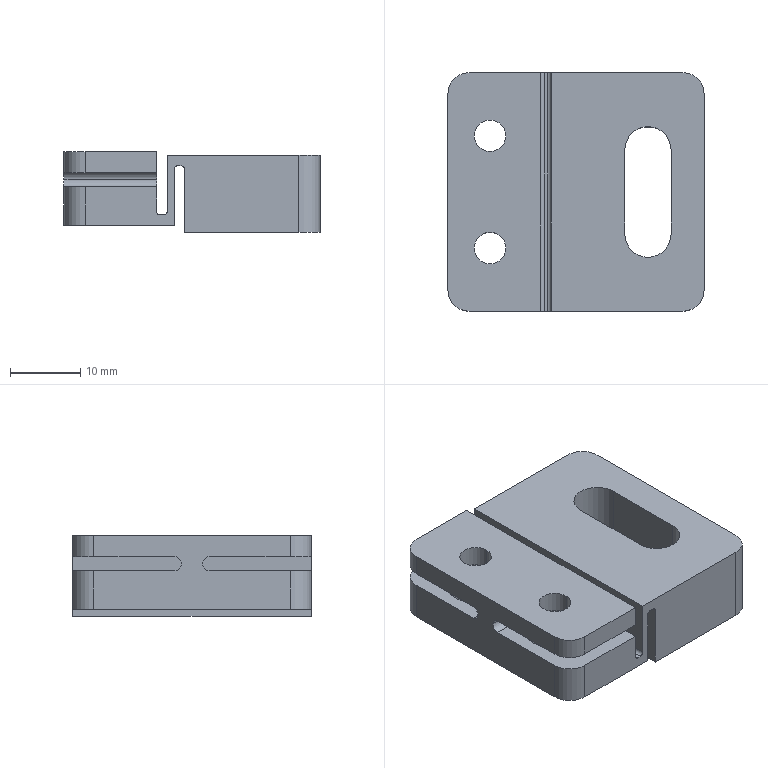Part | SolidWorks | features ICE 13, MoveFace 5, Fillet 3, DelFace 2, Extrusion 1, PLine 1 | 1 solid | 46 faces | box 36.5 x 34 x 11.5 mm | volume 9581 mm3 | cylinder 24 | plane 22 | commonest cylinder face diameters 6 x6 1 x4 2 x4 4.5 x4 8.5 x4 6.6 x2
STEP:
#1=CARTESIAN_POINT('',(-4.75,8.,6.5));
#2=VERTEX_POINT('',#1);
#3=CARTESIAN_POINT('',(-13.25,8.,6.5));
#4=VERTEX_POINT('',#3);
#5=CARTESIAN_POINT('',(-9.,8.,6.5));
#6=DIRECTION('',(0.,0.,-1.));
#7=DIRECTION('',(-1.,0.,0.));
#8=AXIS2_PLACEMENT_3D('',#5,#6,#7);
#9=CIRCLE('',#8,4.25);
#10=EDGE_CURVE('',#2,#4,#9,.T.);
#11=ORIENTED_EDGE('',*,*,#10,.F.);
#12=CARTESIAN_POINT('',(-4.75,8.,1.));
#13=VERTEX_POINT('',#12);
#14=CARTESIAN_POINT('',(-4.75,8.,7.5));
#15=DIRECTION('',(0.,0.,-1.));
#16=VECTOR('',#15,1000.);
#17=LINE('',#14,#16);
#18=EDGE_CURVE('',#2,#13,#17,.T.);
#19=ORIENTED_EDGE('',*,*,#18,.T.);
#20=CARTESIAN_POINT('',(-13.25,8.,1.));
#21=VERTEX_POINT('',#20);
#22=CARTESIAN_POINT('',(-9.,8.,1.));
#23=DIRECTION('',(0.,0.,-1.));
#24=DIRECTION('',(-1.,0.,0.));
#25=AXIS2_PLACEMENT_3D('',#22,#23,#24);
#26=CIRCLE('',#25,4.25);
#27=EDGE_CURVE('',#13,#21,#26,.T.);
#28=ORIENTED_EDGE('',*,*,#27,.T.);
#29=CARTESIAN_POINT('',(-13.25,8.,7.5));
#30=DIRECTION('',(0.,0.,-1.));
#31=VECTOR('',#30,1000.);
#32=LINE('',#29,#31);
#33=EDGE_CURVE('',#4,#21,#32,.T.);
#34=ORIENTED_EDGE('',*,*,#33,.F.);
#35=EDGE_LOOP('',(#11,#19,#28,#34));
#36=FACE_OUTER_BOUND('',#35,.T.);
#37=CARTESIAN_POINT('',(-9.,8.,7.5));
#38=DIRECTION('',(0.,0.,-1.));
#39=DIRECTION('',(-1.,0.,0.));
#40=AXIS2_PLACEMENT_3D('',#37,#38,#39);
#41=CYLINDRICAL_SURFACE('',#40,4.25);
#42=ADVANCED_FACE('',(#36),#41,.F.);
#43=CARTESIAN_POINT('',(-4.75,-8.,6.5));
#44=VERTEX_POINT('',#43);
#45=CARTESIAN_POINT('',(-13.25,-8.,6.5));
#46=VERTEX_POINT('',#45);
#47=CARTESIAN_POINT('',(-9.,-8.,6.5));
#48=DIRECTION('',(0.,0.,-1.));
#49=DIRECTION('',(-1.,0.,0.));
#50=AXIS2_PLACEMENT_3D('',#47,#48,#49);
#51=CIRCLE('',#50,4.25);
#52=EDGE_CURVE('',#44,#46,#51,.T.);
#53=ORIENTED_EDGE('',*,*,#52,.F.);
#54=CARTESIAN_POINT('',(-4.75,-8.,1.));
#55=VERTEX_POINT('',#54);
#56=CARTESIAN_POINT('',(-4.75,-8.,7.5));
#57=DIRECTION('',(0.,0.,-1.));
#58=VECTOR('',#57,1000.);
#59=LINE('',#56,#58);
#60=EDGE_CURVE('',#44,#55,#59,.T.);
#61=ORIENTED_EDGE('',*,*,#60,.T.);
#62=CARTESIAN_POINT('',(-13.25,-8.,1.));
#63=VERTEX_POINT('',#62);
#64=CARTESIAN_POINT('',(-9.,-8.,1.));
#65=DIRECTION('',(0.,0.,-1.));
#66=DIRECTION('',(-1.,0.,0.));
#67=AXIS2_PLACEMENT_3D('',#64,#65,#66);
#68=CIRCLE('',#67,4.25);
#69=EDGE_CURVE('',#55,#63,#68,.T.);
#70=ORIENTED_EDGE('',*,*,#69,.T.);
#71=CARTESIAN_POINT('',(-13.25,-8.,7.5));
#72=DIRECTION('',(0.,0.,-1.));
#73=VECTOR('',#72,1000.);
#74=LINE('',#71,#73);
#75=EDGE_CURVE('',#46,#63,#74,.T.);
#76=ORIENTED_EDGE('',*,*,#75,.F.);
#77=EDGE_LOOP('',(#53,#61,#70,#76));
#78=FACE_OUTER_BOUND('',#77,.T.);
#79=CARTESIAN_POINT('',(-9.,-8.,7.5));
#80=DIRECTION('',(0.,0.,-1.));
#81=DIRECTION('',(-1.,0.,0.));
#82=AXIS2_PLACEMENT_3D('',#79,#80,#81);
#83=CYLINDRICAL_SURFACE('',#82,4.25);
#84=ADVANCED_FACE('',(#78),#83,.F.);
#85=CARTESIAN_POINT('',(-11.25,8.,8.5));
#86=VERTEX_POINT('',#85);
#87=CARTESIAN_POINT('',(-6.75,8.,8.5));
#88=VERTEX_POINT('',#87);
#89=CARTESIAN_POINT('',(-9.,8.,8.5));
#90=DIRECTION('',(0.,0.,1.));
#91=DIRECTION('',(0.,-1.,0.));
#92=AXIS2_PLACEMENT_3D('',#89,#90,#91);
#93=CIRCLE('',#92,2.25);
#94=EDGE_CURVE('',#86,#88,#93,.T.);
#95=ORIENTED_EDGE('',*,*,#94,.F.);
#96=CARTESIAN_POINT('',(-11.25,8.,11.5));
#97=VERTEX_POINT('',#96);
#98=CARTESIAN_POINT('',(-11.25,8.,-6.364));
#99=DIRECTION('',(0.,0.,1.));
#100=VECTOR('',#99,1000.);
#101=LINE('',#98,#100);
#102=EDGE_CURVE('',#86,#97,#101,.T.);
#103=ORIENTED_EDGE('',*,*,#102,.T.);
#104=CARTESIAN_POINT('',(-6.75,8.,11.5));
#105=VERTEX_POINT('',#104);
#106=CARTESIAN_POINT('',(-9.,8.,11.5));
#107=DIRECTION('',(0.,0.,1.));
#108=DIRECTION('',(1.,0.,0.));
#109=AXIS2_PLACEMENT_3D('',#106,#107,#108);
#110=CIRCLE('',#109,2.25);
#111=EDGE_CURVE('',#97,#105,#110,.T.);
#112=ORIENTED_EDGE('',*,*,#111,.T.);
#113=CARTESIAN_POINT('',(-6.75,8.,-6.364));
#114=DIRECTION('',(0.,0.,1.));
#115=VECTOR('',#114,1000.);
#116=LINE('',#113,#115);
#117=EDGE_CURVE('',#88,#105,#116,.T.);
#118=ORIENTED_EDGE('',*,*,#117,.F.);
#119=EDGE_LOOP('',(#95,#103,#112,#118));
#120=FACE_OUTER_BOUND('',#119,.T.);
#121=CARTESIAN_POINT('',(-9.,8.,-6.364));
#122=DIRECTION('',(0.,0.,1.));
#123=DIRECTION('',(1.,0.,0.));
#124=AXIS2_PLACEMENT_3D('',#121,#122,#123);
#125=CYLINDRICAL_SURFACE('',#124,2.25);
#126=ADVANCED_FACE('',(#120),#125,.F.);
#127=CARTESIAN_POINT('',(-11.25,-8.,8.5));
#128=VERTEX_POINT('',#127);
#129=CARTESIAN_POINT('',(-6.75,-8.,8.5));
#130=VERTEX_POINT('',#129);
#131=CARTESIAN_POINT('',(-9.,-8.,8.5));
#132=DIRECTION('',(0.,0.,1.));
#133=DIRECTION('',(0.,-1.,0.));
#134=AXIS2_PLACEMENT_3D('',#131,#132,#133);
#135=CIRCLE('',#134,2.25);
#136=EDGE_CURVE('',#128,#130,#135,.T.);
#137=ORIENTED_EDGE('',*,*,#136,.F.);
#138=CARTESIAN_POINT('',(-11.25,-8.,11.5));
#139=VERTEX_POINT('',#138);
#140=CARTESIAN_POINT('',(-11.25,-8.,-6.364));
#141=DIRECTION('',(0.,0.,1.));
#142=VECTOR('',#141,1000.);
#143=LINE('',#140,#142);
#144=EDGE_CURVE('',#128,#139,#143,.T.);
#145=ORIENTED_EDGE('',*,*,#144,.T.);
#146=CARTESIAN_POINT('',(-6.75,-8.,11.5));
#147=VERTEX_POINT('',#146);
#148=CARTESIAN_POINT('',(-9.,-8.,11.5));
#149=DIRECTION('',(0.,0.,1.));
#150=DIRECTION('',(1.,0.,0.));
#151=AXIS2_PLACEMENT_3D('',#148,#149,#150);
#152=CIRCLE('',#151,2.25);
#153=EDGE_CURVE('',#139,#147,#152,.T.);
#154=ORIENTED_EDGE('',*,*,#153,.T.);
#155=CARTESIAN_POINT('',(-6.75,-8.,-6.364));
#156=DIRECTION('',(0.,0.,1.));
#157=VECTOR('',#156,1000.);
#158=LINE('',#155,#157);
#159=EDGE_CURVE('',#130,#147,#158,.T.);
#160=ORIENTED_EDGE('',*,*,#159,.F.);
#161=EDGE_LOOP('',(#137,#145,#154,#160));
#162=FACE_OUTER_BOUND('',#161,.T.);
#163=CARTESIAN_POINT('',(-9.,-8.,-6.364));
#164=DIRECTION('',(0.,0.,1.));
#165=DIRECTION('',(1.,0.,0.));
#166=AXIS2_PLACEMENT_3D('',#163,#164,#165);
#167=CYLINDRICAL_SURFACE('',#166,2.25);
#168=ADVANCED_FACE('',(#162),#167,.F.);
#169=CARTESIAN_POINT('',(-1.8,17.,11.5));
#170=VERTEX_POINT('',#169);
#171=CARTESIAN_POINT('',(-1.8,17.,8.5));
#172=VERTEX_POINT('',#171);
#173=CARTESIAN_POINT('',(-1.8,17.,3.5));
#174=DIRECTION('',(0.,0.,-1.));
#175=VECTOR('',#174,1000.);
#176=LINE('',#173,#175);
#177=EDGE_CURVE('',#170,#172,#176,.T.);
#178=ORIENTED_EDGE('',*,*,#177,.T.);
#179=CARTESIAN_POINT('',(-12.,17.,8.5));
#180=VERTEX_POINT('',#179);
#181=CARTESIAN_POINT('',(17.501,17.,8.5));
#182=DIRECTION('',(-1.,0.,0.));
#183=VECTOR('',#182,1000.);
#184=LINE('',#181,#183);
#185=EDGE_CURVE('',#172,#180,#184,.T.);
#186=ORIENTED_EDGE('',*,*,#185,.T.);
#187=CARTESIAN_POINT('',(-12.,17.,11.5));
#188=VERTEX_POINT('',#187);
#189=CARTESIAN_POINT('',(-12.,17.,11.));
#190=DIRECTION('',(0.,0.,1.));
#191=VECTOR('',#190,1000.);
#192=LINE('',#189,#191);
#193=EDGE_CURVE('',#180,#188,#192,.T.);
#194=ORIENTED_EDGE('',*,*,#193,.T.);
#195=CARTESIAN_POINT('',(-4.5,17.,11.5));
#196=DIRECTION('',(-1.,0.,0.));
#197=VECTOR('',#196,1000.);
#198=LINE('',#195,#197);
#199=EDGE_CURVE('',#170,#188,#198,.T.);
#200=ORIENTED_EDGE('',*,*,#199,.F.);
#201=EDGE_LOOP('',(#178,#186,#194,#200));
#202=FACE_OUTER_BOUND('',#201,.T.);
#203=CARTESIAN_POINT('',(-17.5,17.,11.));
#204=DIRECTION('',(0.,-1.,0.));
#205=DIRECTION('',(0.,0.,-1.));
#206=AXIS2_PLACEMENT_3D('',#203,#204,#205);
#207=PLANE('',#206);
#208=ADVANCED_FACE('',(#202),#207,.F.);
#209=CARTESIAN_POINT('',(-12.,-17.,11.5));
#210=VERTEX_POINT('',#209);
#211=CARTESIAN_POINT('',(-12.,-17.,8.5));
#212=VERTEX_POINT('',#211);
#213=CARTESIAN_POINT('',(-12.,-17.,11.));
#214=DIRECTION('',(0.,0.,-1.));
#215=VECTOR('',#214,1000.);
#216=LINE('',#213,#215);
#217=EDGE_CURVE('',#210,#212,#216,.T.);
#218=ORIENTED_EDGE('',*,*,#217,.T.);
#219=CARTESIAN_POINT('',(-1.8,-17.,8.5));
#220=VERTEX_POINT('',#219);
#221=CARTESIAN_POINT('',(17.501,-17.,8.5));
#222=DIRECTION('',(-1.,0.,0.));
#223=VECTOR('',#222,1000.);
#224=LINE('',#221,#223);
#225=EDGE_CURVE('',#220,#212,#224,.T.);
#226=ORIENTED_EDGE('',*,*,#225,.F.);
#227=CARTESIAN_POINT('',(-1.8,-17.,11.5));
#228=VERTEX_POINT('',#227);
#229=CARTESIAN_POINT('',(-1.8,-17.,3.5));
#230=DIRECTION('',(0.,0.,-1.));
#231=VECTOR('',#230,1000.);
#232=LINE('',#229,#231);
#233=EDGE_CURVE('',#228,#220,#232,.T.);
#234=ORIENTED_EDGE('',*,*,#233,.F.);
#235=CARTESIAN_POINT('',(-4.5,-17.,11.5));
#236=DIRECTION('',(1.,0.,0.));
#237=VECTOR('',#236,1000.);
#238=LINE('',#235,#237);
#239=EDGE_CURVE('',#210,#228,#238,.T.);
#240=ORIENTED_EDGE('',*,*,#239,.F.);
#241=EDGE_LOOP('',(#218,#226,#234,#240));
#242=FACE_OUTER_BOUND('',#241,.T.);
#243=CARTESIAN_POINT('',(-17.5,-17.,11.));
#244=DIRECTION('',(0.,1.,0.));
#245=DIRECTION('',(0.,0.,1.));
#246=AXIS2_PLACEMENT_3D('',#243,#244,#245);
#247=PLANE('',#246);
#248=ADVANCED_FACE('',(#242),#247,.F.);
#249=CARTESIAN_POINT('',(-15.,-14.,8.5));
#250=VERTEX_POINT('',#249);
#251=CARTESIAN_POINT('',(-12.,-14.,8.5));
#252=DIRECTION('',(0.,0.,1.));
#253=DIRECTION('',(0.,-1.,0.));
#254=AXIS2_PLACEMENT_3D('',#251,#252,#253);
#255=CIRCLE('',#254,3.);
#256=EDGE_CURVE('',#250,#212,#255,.T.);
#257=ORIENTED_EDGE('',*,*,#256,.T.);
#258=ORIENTED_EDGE('',*,*,#217,.F.);
#259=CARTESIAN_POINT('',(-15.,-14.,11.5));
#260=VERTEX_POINT('',#259);
#261=CARTESIAN_POINT('',(-12.,-14.,11.5));
#262=DIRECTION('',(0.,0.,1.));
#263=DIRECTION('',(-1.,0.,0.));
#264=AXIS2_PLACEMENT_3D('',#261,#262,#263);
#265=CIRCLE('',#264,3.);
#266=EDGE_CURVE('',#260,#210,#265,.T.);
#267=ORIENTED_EDGE('',*,*,#266,.F.);
#268=CARTESIAN_POINT('',(-15.,-14.,11.));
#269=DIRECTION('',(0.,0.,1.));
#270=VECTOR('',#269,1000.);
#271=LINE('',#268,#270);
#272=EDGE_CURVE('',#250,#260,#271,.T.);
#273=ORIENTED_EDGE('',*,*,#272,.F.);
#274=EDGE_LOOP('',(#257,#258,#267,#273));
#275=FACE_OUTER_BOUND('',#274,.T.);
#276=CARTESIAN_POINT('',(-12.,-14.,11.));
#277=DIRECTION('',(0.,0.,-1.));
#278=DIRECTION('',(-1.,0.,0.));
#279=AXIS2_PLACEMENT_3D('',#276,#277,#278);
#280=CYLINDRICAL_SURFACE('',#279,3.);
#281=ADVANCED_FACE('',(#275),#280,.T.);
#282=CARTESIAN_POINT('',(-15.,14.,8.5));
#283=VERTEX_POINT('',#282);
#284=CARTESIAN_POINT('',(-12.,14.,8.5));
#285=DIRECTION('',(0.,0.,1.));
#286=DIRECTION('',(0.,-1.,0.));
#287=AXIS2_PLACEMENT_3D('',#284,#285,#286);
#288=CIRCLE('',#287,3.);
#289=EDGE_CURVE('',#180,#283,#288,.T.);
#290=ORIENTED_EDGE('',*,*,#289,.T.);
#291=CARTESIAN_POINT('',(-15.,14.,11.5));
#292=VERTEX_POINT('',#291);
#293=CARTESIAN_POINT('',(-15.,14.,11.));
#294=DIRECTION('',(0.,0.,-1.));
#295=VECTOR('',#294,1000.);
#296=LINE('',#293,#295);
#297=EDGE_CURVE('',#292,#283,#296,.T.);
#298=ORIENTED_EDGE('',*,*,#297,.F.);
#299=CARTESIAN_POINT('',(-12.,14.,11.5));
#300=DIRECTION('',(0.,0.,1.));
#301=DIRECTION('',(-1.,0.,0.));
#302=AXIS2_PLACEMENT_3D('',#299,#300,#301);
#303=CIRCLE('',#302,3.);
#304=EDGE_CURVE('',#188,#292,#303,.T.);
#305=ORIENTED_EDGE('',*,*,#304,.F.);
#306=ORIENTED_EDGE('',*,*,#193,.F.);
#307=EDGE_LOOP('',(#290,#298,#305,#306));
#308=FACE_OUTER_BOUND('',#307,.T.);
#309=CARTESIAN_POINT('',(-12.,14.,11.));
#310=DIRECTION('',(0.,0.,-1.));
#311=DIRECTION('',(-1.,0.,0.));
#312=AXIS2_PLACEMENT_3D('',#309,#310,#311);
#313=CYLINDRICAL_SURFACE('',#312,3.);
#314=ADVANCED_FACE('',(#308),#313,.T.);
#315=CARTESIAN_POINT('',(10.2,6.,11.));
#316=VERTEX_POINT('',#315);
#317=CARTESIAN_POINT('',(10.2,-6.,11.));
#318=VERTEX_POINT('',#317);
#319=CARTESIAN_POINT('',(10.2,-6.,11.));
#320=DIRECTION('',(0.,-1.,0.));
#321=VECTOR('',#320,1000.);
#322=LINE('',#319,#321);
#323=EDGE_CURVE('',#316,#318,#322,.T.);
#324=ORIENTED_EDGE('',*,*,#323,.F.);
#325=CARTESIAN_POINT('',(16.8,6.,11.));
#326=VERTEX_POINT('',#325);
#327=CARTESIAN_POINT('',(13.5,6.,11.));
#328=DIRECTION('',(0.,0.,1.));
#329=DIRECTION('',(-1.,0.,0.));
#330=AXIS2_PLACEMENT_3D('',#327,#328,#329);
#331=CIRCLE('',#330,3.3);
#332=EDGE_CURVE('',#326,#316,#331,.T.);
#333=ORIENTED_EDGE('',*,*,#332,.F.);
#334=CARTESIAN_POINT('',(16.8,-6.,11.));
#335=VERTEX_POINT('',#334);
#336=CARTESIAN_POINT('',(16.8,-6.,11.));
#337=DIRECTION('',(0.,1.,0.));
#338=VECTOR('',#337,1000.);
#339=LINE('',#336,#338);
#340=EDGE_CURVE('',#335,#326,#339,.T.);
#341=ORIENTED_EDGE('',*,*,#340,.F.);
#342=CARTESIAN_POINT('',(13.5,-6.,11.));
#343=DIRECTION('',(0.,0.,1.));
#344=DIRECTION('',(-1.,0.,0.));
#345=AXIS2_PLACEMENT_3D('',#342,#343,#344);
#346=CIRCLE('',#345,3.3);
#347=EDGE_CURVE('',#318,#335,#346,.T.);
#348=ORIENTED_EDGE('',*,*,#347,.F.);
#349=EDGE_LOOP('',(#324,#333,#341,#348));
#350=FACE_BOUND('',#349,.T.);
#351=CARTESIAN_POINT('',(18.5,17.,11.));
#352=VERTEX_POINT('',#351);
#353=CARTESIAN_POINT('',(-0.3,17.,11.));
#354=VERTEX_POINT('',#353);
#355=CARTESIAN_POINT('',(-17.5,17.,11.));
#356=DIRECTION('',(-1.,0.,0.));
#357=VECTOR('',#356,1000.);
#358=LINE('',#355,#357);
#359=EDGE_CURVE('',#352,#354,#358,.T.);
#360=ORIENTED_EDGE('',*,*,#359,.T.);
#361=CARTESIAN_POINT('',(-0.3,-17.,11.));
#362=VERTEX_POINT('',#361);
#363=CARTESIAN_POINT('',(-0.3,17.,11.));
#364=DIRECTION('',(0.,-1.,0.));
#365=VECTOR('',#364,1000.);
#366=LINE('',#363,#365);
#367=EDGE_CURVE('',#354,#362,#366,.T.);
#368=ORIENTED_EDGE('',*,*,#367,.T.);
#369=CARTESIAN_POINT('',(18.5,-17.,11.));
#370=VERTEX_POINT('',#369);
#371=CARTESIAN_POINT('',(-17.5,-17.,11.));
#372=DIRECTION('',(1.,0.,0.));
#373=VECTOR('',#372,1000.);
#374=LINE('',#371,#373);
#375=EDGE_CURVE('',#362,#370,#374,.T.);
#376=ORIENTED_EDGE('',*,*,#375,.T.);
#377=CARTESIAN_POINT('',(21.5,-14.,11.));
#378=VERTEX_POINT('',#377);
#379=CARTESIAN_POINT('',(18.5,-14.,11.));
#380=DIRECTION('',(0.,0.,1.));
#381=DIRECTION('',(-1.,0.,0.));
#382=AXIS2_PLACEMENT_3D('',#379,#380,#381);
#383=CIRCLE('',#382,3.);
#384=EDGE_CURVE('',#370,#378,#383,.T.);
#385=ORIENTED_EDGE('',*,*,#384,.T.);
#386=CARTESIAN_POINT('',(21.5,14.,11.));
#387=VERTEX_POINT('',#386);
#388=CARTESIAN_POINT('',(21.5,17.,11.));
#389=DIRECTION('',(0.,-1.,0.));
#390=VECTOR('',#389,1000.);
#391=LINE('',#388,#390);
#392=EDGE_CURVE('',#387,#378,#391,.T.);
#393=ORIENTED_EDGE('',*,*,#392,.F.);
#394=CARTESIAN_POINT('',(18.5,14.,11.));
#395=DIRECTION('',(0.,0.,1.));
#396=DIRECTION('',(-1.,0.,0.));
#397=AXIS2_PLACEMENT_3D('',#394,#395,#396);
#398=CIRCLE('',#397,3.);
#399=EDGE_CURVE('',#387,#352,#398,.T.);
#400=ORIENTED_EDGE('',*,*,#399,.T.);
#401=EDGE_LOOP('',(#360,#368,#376,#385,#393,#400));
#402=FACE_OUTER_BOUND('',#401,.T.);
#403=CARTESIAN_POINT('',(-0.1,37.,11.));
#404=DIRECTION('',(0.,0.,-1.));
#405=DIRECTION('',(-1.,0.,0.));
#406=AXIS2_PLACEMENT_3D('',#403,#404,#405);
#407=PLANE('',#406);
#408=ADVANCED_FACE('',(#350,#402),#407,.F.);
#409=CARTESIAN_POINT('',(-12.,17.,1.));
#410=VERTEX_POINT('',#409);
#411=CARTESIAN_POINT('',(-12.,17.,6.5));
#412=VERTEX_POINT('',#411);
#413=CARTESIAN_POINT('',(-12.,17.,11.));
#414=DIRECTION('',(0.,0.,1.));
#415=VECTOR('',#414,1000.);
#416=LINE('',#413,#415);
#417=EDGE_CURVE('',#410,#412,#416,.T.);
#418=ORIENTED_EDGE('',*,*,#417,.T.);
#419=CARTESIAN_POINT('',(-1.8,17.,6.5));
#420=VERTEX_POINT('',#419);
#421=CARTESIAN_POINT('',(17.501,17.,6.5));
#422=DIRECTION('',(-1.,0.,0.));
#423=VECTOR('',#422,1000.);
#424=LINE('',#421,#423);
#425=EDGE_CURVE('',#420,#412,#424,.T.);
#426=ORIENTED_EDGE('',*,*,#425,.F.);
#427=CARTESIAN_POINT('',(-1.8,17.,3.));
#428=VERTEX_POINT('',#427);
#429=CARTESIAN_POINT('',(-1.8,17.,3.5));
#430=DIRECTION('',(0.,0.,-1.));
#431=VECTOR('',#430,1000.);
#432=LINE('',#429,#431);
#433=EDGE_CURVE('',#420,#428,#432,.T.);
#434=ORIENTED_EDGE('',*,*,#433,.T.);
#435=CARTESIAN_POINT('',(-1.3,17.,2.5));
#436=VERTEX_POINT('',#435);
#437=CARTESIAN_POINT('',(-1.3,17.,3.));
#438=DIRECTION('',(0.,-1.,0.));
#439=DIRECTION('',(0.,0.,-1.));
#440=AXIS2_PLACEMENT_3D('',#437,#438,#439);
#441=CIRCLE('',#440,0.5);
#442=EDGE_CURVE('',#428,#436,#441,.T.);
#443=ORIENTED_EDGE('',*,*,#442,.T.);
#444=CARTESIAN_POINT('',(-0.8,17.,2.5));
#445=VERTEX_POINT('',#444);
#446=CARTESIAN_POINT('',(-0.3,17.,2.5));
#447=DIRECTION('',(1.,0.,0.));
#448=VECTOR('',#447,1000.);
#449=LINE('',#446,#448);
#450=EDGE_CURVE('',#436,#445,#449,.T.);
#451=ORIENTED_EDGE('',*,*,#450,.T.);
#452=CARTESIAN_POINT('',(-0.3,17.,3.));
#453=VERTEX_POINT('',#452);
#454=CARTESIAN_POINT('',(-0.8,17.,3.));
#455=DIRECTION('',(0.,-1.,0.));
#456=DIRECTION('',(0.,0.,-1.));
#457=AXIS2_PLACEMENT_3D('',#454,#455,#456);
#458=CIRCLE('',#457,0.5);
#459=EDGE_CURVE('',#445,#453,#458,.T.);
#460=ORIENTED_EDGE('',*,*,#459,.T.);
#461=CARTESIAN_POINT('',(-0.3,17.,11.));
#462=DIRECTION('',(0.,0.,1.));
#463=VECTOR('',#462,1000.);
#464=LINE('',#461,#463);
#465=EDGE_CURVE('',#453,#354,#464,.T.);
#466=ORIENTED_EDGE('',*,*,#465,.T.);
#467=ORIENTED_EDGE('',*,*,#359,.F.);
#468=CARTESIAN_POINT('',(18.5,17.,0.));
#469=VERTEX_POINT('',#468);
#470=CARTESIAN_POINT('',(18.5,17.,11.));
#471=DIRECTION('',(0.,0.,-1.));
#472=VECTOR('',#471,1000.);
#473=LINE('',#470,#472);
#474=EDGE_CURVE('',#352,#469,#473,.T.);
#475=ORIENTED_EDGE('',*,*,#474,.T.);
#476=CARTESIAN_POINT('',(2.2,17.,0.));
#477=VERTEX_POINT('',#476);
#478=CARTESIAN_POINT('',(-17.5,17.,0.));
#479=DIRECTION('',(-1.,0.,0.));
#480=VECTOR('',#479,1000.);
#481=LINE('',#478,#480);
#482=EDGE_CURVE('',#469,#477,#481,.T.);
#483=ORIENTED_EDGE('',*,*,#482,.T.);
#484=CARTESIAN_POINT('',(2.2,17.,9.));
#485=VERTEX_POINT('',#484);
#486=CARTESIAN_POINT('',(2.2,17.,-9.));
#487=DIRECTION('',(0.,0.,1.));
#488=VECTOR('',#487,1000.);
#489=LINE('',#486,#488);
#490=EDGE_CURVE('',#477,#485,#489,.T.);
#491=ORIENTED_EDGE('',*,*,#490,.T.);
#492=CARTESIAN_POINT('',(1.7,17.,9.5));
#493=VERTEX_POINT('',#492);
#494=CARTESIAN_POINT('',(1.7,17.,9.));
#495=DIRECTION('',(0.,-1.,0.));
#496=DIRECTION('',(0.,0.,-1.));
#497=AXIS2_PLACEMENT_3D('',#494,#495,#496);
#498=CIRCLE('',#497,0.5);
#499=EDGE_CURVE('',#485,#493,#498,.T.);
#500=ORIENTED_EDGE('',*,*,#499,.T.);
#501=CARTESIAN_POINT('',(1.2,17.,9.5));
#502=VERTEX_POINT('',#501);
#503=CARTESIAN_POINT('',(2.2,17.,9.5));
#504=DIRECTION('',(-1.,0.,0.));
#505=VECTOR('',#504,1000.);
#506=LINE('',#503,#505);
#507=EDGE_CURVE('',#493,#502,#506,.T.);
#508=ORIENTED_EDGE('',*,*,#507,.T.);
#509=CARTESIAN_POINT('',(0.7,17.,9.));
#510=VERTEX_POINT('',#509);
#511=CARTESIAN_POINT('',(1.2,17.,9.));
#512=DIRECTION('',(0.,-1.,0.));
#513=DIRECTION('',(0.,0.,-1.));
#514=AXIS2_PLACEMENT_3D('',#511,#512,#513);
#515=CIRCLE('',#514,0.5);
#516=EDGE_CURVE('',#502,#510,#515,.T.);
#517=ORIENTED_EDGE('',*,*,#516,.T.);
#518=CARTESIAN_POINT('',(0.7,17.,1.));
#519=VERTEX_POINT('',#518);
#520=CARTESIAN_POINT('',(0.7,17.,9.5));
#521=DIRECTION('',(0.,0.,-1.));
#522=VECTOR('',#521,1000.);
#523=LINE('',#520,#522);
#524=EDGE_CURVE('',#510,#519,#523,.T.);
#525=ORIENTED_EDGE('',*,*,#524,.T.);
#526=CARTESIAN_POINT('',(-17.5,17.,1.));
#527=DIRECTION('',(1.,0.,0.));
#528=VECTOR('',#527,1000.);
#529=LINE('',#526,#528);
#530=EDGE_CURVE('',#410,#519,#529,.T.);
#531=ORIENTED_EDGE('',*,*,#530,.F.);
#532=EDGE_LOOP('',(#418,#426,#434,#443,#451,#460,#466,#467,#475,#483,#491,#500,#508,#517,#525,#531));
#533=FACE_OUTER_BOUND('',#532,.T.);
#534=CARTESIAN_POINT('',(-17.5,17.,11.));
#535=DIRECTION('',(0.,-1.,0.));
#536=DIRECTION('',(0.,0.,-1.));
#537=AXIS2_PLACEMENT_3D('',#534,#535,#536);
#538=PLANE('',#537);
#539=ADVANCED_FACE('',(#533),#538,.F.);
#540=CARTESIAN_POINT('',(-1.8,-17.,6.5));
#541=VERTEX_POINT('',#540);
#542=CARTESIAN_POINT('',(-1.8,-17.,3.));
#543=VERTEX_POINT('',#542);
#544=CARTESIAN_POINT('',(-1.8,-17.,3.5));
#545=DIRECTION('',(0.,0.,-1.));
#546=VECTOR('',#545,1000.);
#547=LINE('',#544,#546);
#548=EDGE_CURVE('',#541,#543,#547,.T.);
#549=ORIENTED_EDGE('',*,*,#548,.F.);
#550=CARTESIAN_POINT('',(-12.,-17.,6.5));
#551=VERTEX_POINT('',#550);
#552=CARTESIAN_POINT('',(17.501,-17.,6.5));
#553=DIRECTION('',(-1.,0.,0.));
#554=VECTOR('',#553,1000.);
#555=LINE('',#552,#554);
#556=EDGE_CURVE('',#541,#551,#555,.T.);
#557=ORIENTED_EDGE('',*,*,#556,.T.);
#558=CARTESIAN_POINT('',(-12.,-17.,1.));
#559=VERTEX_POINT('',#558);
#560=CARTESIAN_POINT('',(-12.,-17.,11.));
#561=DIRECTION('',(0.,0.,-1.));
#562=VECTOR('',#561,1000.);
#563=LINE('',#560,#562);
#564=EDGE_CURVE('',#551,#559,#563,.T.);
#565=ORIENTED_EDGE('',*,*,#564,.T.);
#566=CARTESIAN_POINT('',(0.7,-17.,1.));
#567=VERTEX_POINT('',#566);
#568=CARTESIAN_POINT('',(-17.5,-17.,1.));
#569=DIRECTION('',(-1.,0.,0.));
#570=VECTOR('',#569,1000.);
#571=LINE('',#568,#570);
#572=EDGE_CURVE('',#567,#559,#571,.T.);
#573=ORIENTED_EDGE('',*,*,#572,.F.);
#574=CARTESIAN_POINT('',(0.7,-17.,9.));
#575=VERTEX_POINT('',#574);
#576=CARTESIAN_POINT('',(0.7,-17.,9.5));
#577=DIRECTION('',(0.,0.,-1.));
#578=VECTOR('',#577,1000.);
#579=LINE('',#576,#578);
#580=EDGE_CURVE('',#575,#567,#579,.T.);
#581=ORIENTED_EDGE('',*,*,#580,.F.);
#582=CARTESIAN_POINT('',(1.2,-17.,9.5));
#583=VERTEX_POINT('',#582);
#584=CARTESIAN_POINT('',(1.2,-17.,9.));
#585=DIRECTION('',(0.,1.,0.));
#586=DIRECTION('',(0.,0.,1.));
#587=AXIS2_PLACEMENT_3D('',#584,#585,#586);
#588=CIRCLE('',#587,0.5);
#589=EDGE_CURVE('',#575,#583,#588,.T.);
#590=ORIENTED_EDGE('',*,*,#589,.T.);
#591=CARTESIAN_POINT('',(1.7,-17.,9.5));
#592=VERTEX_POINT('',#591);
#593=CARTESIAN_POINT('',(2.2,-17.,9.5));
#594=DIRECTION('',(-1.,0.,0.));
#595=VECTOR('',#594,1000.);
#596=LINE('',#593,#595);
#597=EDGE_CURVE('',#592,#583,#596,.T.);
#598=ORIENTED_EDGE('',*,*,#597,.F.);
#599=CARTESIAN_POINT('',(2.2,-17.,9.));
#600=VERTEX_POINT('',#599);
#601=CARTESIAN_POINT('',(1.7,-17.,9.));
#602=DIRECTION('',(0.,1.,0.));
#603=DIRECTION('',(0.,0.,1.));
#604=AXIS2_PLACEMENT_3D('',#601,#602,#603);
#605=CIRCLE('',#604,0.5);
#606=EDGE_CURVE('',#592,#600,#605,.T.);
#607=ORIENTED_EDGE('',*,*,#606,.T.);
#608=CARTESIAN_POINT('',(2.2,-17.,0.));
#609=VERTEX_POINT('',#608);
#610=CARTESIAN_POINT('',(2.2,-17.,11.));
#611=DIRECTION('',(0.,0.,1.));
#612=VECTOR('',#611,1000.);
#613=LINE('',#610,#612);
#614=EDGE_CURVE('',#609,#600,#613,.T.);
#615=ORIENTED_EDGE('',*,*,#614,.F.);
#616=CARTESIAN_POINT('',(18.5,-17.,0.));
#617=VERTEX_POINT('',#616);
#618=CARTESIAN_POINT('',(-17.5,-17.,0.));
#619=DIRECTION('',(1.,0.,0.));
#620=VECTOR('',#619,1000.);
#621=LINE('',#618,#620);
#622=EDGE_CURVE('',#609,#617,#621,.T.);
#623=ORIENTED_EDGE('',*,*,#622,.T.);
#624=CARTESIAN_POINT('',(18.5,-17.,11.));
#625=DIRECTION('',(0.,0.,1.));
#626=VECTOR('',#625,1000.);
#627=LINE('',#624,#626);
#628=EDGE_CURVE('',#617,#370,#627,.T.);
#629=ORIENTED_EDGE('',*,*,#628,.T.);
#630=ORIENTED_EDGE('',*,*,#375,.F.);
#631=CARTESIAN_POINT('',(-0.3,-17.,3.));
#632=VERTEX_POINT('',#631);
#633=CARTESIAN_POINT('',(-0.3,-17.,11.));
#634=DIRECTION('',(0.,0.,1.));
#635=VECTOR('',#634,1000.);
#636=LINE('',#633,#635);
#637=EDGE_CURVE('',#632,#362,#636,.T.);
#638=ORIENTED_EDGE('',*,*,#637,.F.);
#639=CARTESIAN_POINT('',(-0.8,-17.,2.5));
#640=VERTEX_POINT('',#639);
#641=CARTESIAN_POINT('',(-0.8,-17.,3.));
#642=DIRECTION('',(0.,1.,0.));
#643=DIRECTION('',(0.,0.,1.));
#644=AXIS2_PLACEMENT_3D('',#641,#642,#643);
#645=CIRCLE('',#644,0.5);
#646=EDGE_CURVE('',#632,#640,#645,.T.);
#647=ORIENTED_EDGE('',*,*,#646,.T.);
#648=CARTESIAN_POINT('',(-1.3,-17.,2.5));
#649=VERTEX_POINT('',#648);
#650=CARTESIAN_POINT('',(-0.3,-17.,2.5));
#651=DIRECTION('',(1.,0.,0.));
#652=VECTOR('',#651,1000.);
#653=LINE('',#650,#652);
#654=EDGE_CURVE('',#649,#640,#653,.T.);
#655=ORIENTED_EDGE('',*,*,#654,.F.);
#656=CARTESIAN_POINT('',(-1.3,-17.,3.));
#657=DIRECTION('',(0.,1.,0.));
#658=DIRECTION('',(0.,0.,1.));
#659=AXIS2_PLACEMENT_3D('',#656,#657,#658);
#660=CIRCLE('',#659,0.5);
#661=EDGE_CURVE('',#649,#543,#660,.T.);
#662=ORIENTED_EDGE('',*,*,#661,.T.);
#663=EDGE_LOOP('',(#549,#557,#565,#573,#581,#590,#598,#607,#615,#623,#629,#630,#638,#647,#655,#662));
#664=FACE_OUTER_BOUND('',#663,.T.);
#665=CARTESIAN_POINT('',(-17.5,-17.,11.));
#666=DIRECTION('',(0.,1.,0.));
#667=DIRECTION('',(0.,0.,1.));
#668=AXIS2_PLACEMENT_3D('',#665,#666,#667);
#669=PLANE('',#668);
#670=ADVANCED_FACE('',(#664),#669,.F.);
#671=CARTESIAN_POINT('',(10.2,-6.,0.));
#672=VERTEX_POINT('',#671);
#673=CARTESIAN_POINT('',(10.2,6.,0.));
#674=VERTEX_POINT('',#673);
#675=CARTESIAN_POINT('',(10.2,-6.,0.));
#676=DIRECTION('',(0.,1.,0.));
#677=VECTOR('',#676,1000.);
#678=LINE('',#675,#677);
#679=EDGE_CURVE('',#672,#674,#678,.T.);
#680=ORIENTED_EDGE('',*,*,#679,.F.);
#681=CARTESIAN_POINT('',(16.8,-6.,0.));
#682=VERTEX_POINT('',#681);
#683=CARTESIAN_POINT('',(13.5,-6.,0.));
#684=DIRECTION('',(0.,0.,-1.));
#685=DIRECTION('',(1.,0.,0.));
#686=AXIS2_PLACEMENT_3D('',#683,#684,#685);
#687=CIRCLE('',#686,3.3);
#688=EDGE_CURVE('',#682,#672,#687,.T.);
#689=ORIENTED_EDGE('',*,*,#688,.F.);
#690=CARTESIAN_POINT('',(16.8,6.,0.));
#691=VERTEX_POINT('',#690);
#692=CARTESIAN_POINT('',(16.8,-6.,0.));
#693=DIRECTION('',(0.,-1.,0.));
#694=VECTOR('',#693,1000.);
#695=LINE('',#692,#694);
#696=EDGE_CURVE('',#691,#682,#695,.T.);
#697=ORIENTED_EDGE('',*,*,#696,.F.);
#698=CARTESIAN_POINT('',(13.5,6.,0.));
#699=DIRECTION('',(0.,0.,-1.));
#700=DIRECTION('',(1.,0.,0.));
#701=AXIS2_PLACEMENT_3D('',#698,#699,#700);
#702=CIRCLE('',#701,3.3);
#703=EDGE_CURVE('',#674,#691,#702,.T.);
#704=ORIENTED_EDGE('',*,*,#703,.F.);
#705=EDGE_LOOP('',(#680,#689,#697,#704));
#706=FACE_BOUND('',#705,.T.);
#707=CARTESIAN_POINT('',(2.2,0.,0.));
#708=DIRECTION('',(0.,-1.,0.));
#709=VECTOR('',#708,1000.);
#710=LINE('',#707,#709);
#711=EDGE_CURVE('',#477,#609,#710,.T.);
#712=ORIENTED_EDGE('',*,*,#711,.F.);
#713=ORIENTED_EDGE('',*,*,#482,.F.);
#714=CARTESIAN_POINT('',(21.5,14.,0.));
#715=VERTEX_POINT('',#714);
#716=CARTESIAN_POINT('',(18.5,14.,0.));
#717=DIRECTION('',(0.,0.,-1.));
#718=DIRECTION('',(1.,0.,0.));
#719=AXIS2_PLACEMENT_3D('',#716,#717,#718);
#720=CIRCLE('',#719,3.);
#721=EDGE_CURVE('',#469,#715,#720,.T.);
#722=ORIENTED_EDGE('',*,*,#721,.T.);
#723=CARTESIAN_POINT('',(21.5,-14.,0.));
#724=VERTEX_POINT('',#723);
#725=CARTESIAN_POINT('',(21.5,17.,0.));
#726=DIRECTION('',(0.,1.,0.));
#727=VECTOR('',#726,1000.);
#728=LINE('',#725,#727);
#729=EDGE_CURVE('',#724,#715,#728,.T.);
#730=ORIENTED_EDGE('',*,*,#729,.F.);
#731=CARTESIAN_POINT('',(18.5,-14.,0.));
#732=DIRECTION('',(0.,0.,-1.));
#733=DIRECTION('',(1.,0.,0.));
#734=AXIS2_PLACEMENT_3D('',#731,#732,#733);
#735=CIRCLE('',#734,3.);
#736=EDGE_CURVE('',#724,#617,#735,.T.);
#737=ORIENTED_EDGE('',*,*,#736,.T.);
#738=ORIENTED_EDGE('',*,*,#622,.F.);
#739=EDGE_LOOP('',(#712,#713,#722,#730,#737,#738));
#740=FACE_OUTER_BOUND('',#739,.T.);
#741=CARTESIAN_POINT('',(0.,0.,0.));
#742=DIRECTION('',(0.,0.,1.));
#743=DIRECTION('',(1.,0.,0.));
#744=AXIS2_PLACEMENT_3D('',#741,#742,#743);
#745=PLANE('',#744);
#746=ADVANCED_FACE('',(#706,#740),#745,.F.);
#747=ORIENTED_EDGE('',*,*,#144,.F.);
#748=CARTESIAN_POINT('',(-9.,-8.,8.5));
#749=DIRECTION('',(0.,0.,1.));
#750=DIRECTION('',(0.,-1.,0.));
#751=AXIS2_PLACEMENT_3D('',#748,#749,#750);
#752=CIRCLE('',#751,2.25);
#753=EDGE_CURVE('',#130,#128,#752,.T.);
#754=ORIENTED_EDGE('',*,*,#753,.F.);
#755=ORIENTED_EDGE('',*,*,#159,.T.);
#756=CARTESIAN_POINT('',(-9.,-8.,11.5));
#757=DIRECTION('',(0.,0.,1.));
#758=DIRECTION('',(1.,0.,0.));
#759=AXIS2_PLACEMENT_3D('',#756,#757,#758);
#760=CIRCLE('',#759,2.25);
#761=EDGE_CURVE('',#147,#139,#760,.T.);
#762=ORIENTED_EDGE('',*,*,#761,.T.);
#763=EDGE_LOOP('',(#747,#754,#755,#762));
#764=FACE_OUTER_BOUND('',#763,.T.);
#765=CARTESIAN_POINT('',(-9.,-8.,-6.364));
#766=DIRECTION('',(0.,0.,1.));
#767=DIRECTION('',(1.,0.,0.));
#768=AXIS2_PLACEMENT_3D('',#765,#766,#767);
#769=CYLINDRICAL_SURFACE('',#768,2.25);
#770=ADVANCED_FACE('',(#764),#769,.F.);
#771=ORIENTED_EDGE('',*,*,#102,.F.);
#772=CARTESIAN_POINT('',(-9.,8.,8.5));
#773=DIRECTION('',(0.,0.,1.));
#774=DIRECTION('',(0.,-1.,0.));
#775=AXIS2_PLACEMENT_3D('',#772,#773,#774);
#776=CIRCLE('',#775,2.25);
#777=EDGE_CURVE('',#88,#86,#776,.T.);
#778=ORIENTED_EDGE('',*,*,#777,.F.);
#779=ORIENTED_EDGE('',*,*,#117,.T.);
#780=CARTESIAN_POINT('',(-9.,8.,11.5));
#781=DIRECTION('',(0.,0.,1.));
#782=DIRECTION('',(1.,0.,0.));
#783=AXIS2_PLACEMENT_3D('',#780,#781,#782);
#784=CIRCLE('',#783,2.25);
#785=EDGE_CURVE('',#105,#97,#784,.T.);
#786=ORIENTED_EDGE('',*,*,#785,.T.);
#787=EDGE_LOOP('',(#771,#778,#779,#786));
#788=FACE_OUTER_BOUND('',#787,.T.);
#789=CARTESIAN_POINT('',(-9.,8.,-6.364));
#790=DIRECTION('',(0.,0.,1.));
#791=DIRECTION('',(1.,0.,0.));
#792=AXIS2_PLACEMENT_3D('',#789,#790,#791);
#793=CYLINDRICAL_SURFACE('',#792,2.25);
#794=ADVANCED_FACE('',(#788),#793,.F.);
#795=ORIENTED_EDGE('',*,*,#297,.T.);
#796=CARTESIAN_POINT('',(-15.,2.5,8.5));
#797=VERTEX_POINT('',#796);
#798=CARTESIAN_POINT('',(-15.,17.,8.5));
#799=DIRECTION('',(0.,1.,0.));
#800=VECTOR('',#799,1000.);
#801=LINE('',#798,#800);
#802=EDGE_CURVE('',#797,#283,#801,.T.);
#803=ORIENTED_EDGE('',*,*,#802,.F.);
#804=CARTESIAN_POINT('',(-15.,1.5,7.5));
#805=VERTEX_POINT('',#804);
#806=CARTESIAN_POINT('',(-15.,2.5,7.5));
#807=DIRECTION('',(1.,0.,0.));
#808=DIRECTION('',(0.,1.,0.));
#809=AXIS2_PLACEMENT_3D('',#806,#807,#808);
#810=CIRCLE('',#809,1.);
#811=EDGE_CURVE('',#797,#805,#810,.T.);
#812=ORIENTED_EDGE('',*,*,#811,.T.);
#813=CARTESIAN_POINT('',(-15.,2.5,6.5));
#814=VERTEX_POINT('',#813);
#815=CARTESIAN_POINT('',(-15.,2.5,7.5));
#816=DIRECTION('',(1.,0.,0.));
#817=DIRECTION('',(0.,1.,0.));
#818=AXIS2_PLACEMENT_3D('',#815,#816,#817);
#819=CIRCLE('',#818,1.);
#820=EDGE_CURVE('',#805,#814,#819,.T.);
#821=ORIENTED_EDGE('',*,*,#820,.T.);
#822=CARTESIAN_POINT('',(-15.,14.,6.5));
#823=VERTEX_POINT('',#822);
#824=CARTESIAN_POINT('',(-15.,17.,6.5));
#825=DIRECTION('',(0.,-1.,0.));
#826=VECTOR('',#825,1000.);
#827=LINE('',#824,#826);
#828=EDGE_CURVE('',#823,#814,#827,.T.);
#829=ORIENTED_EDGE('',*,*,#828,.F.);
#830=CARTESIAN_POINT('',(-15.,14.,1.));
#831=VERTEX_POINT('',#830);
#832=CARTESIAN_POINT('',(-15.,14.,11.));
#833=DIRECTION('',(0.,0.,-1.));
#834=VECTOR('',#833,1000.);
#835=LINE('',#832,#834);
#836=EDGE_CURVE('',#823,#831,#835,.T.);
#837=ORIENTED_EDGE('',*,*,#836,.T.);
#838=CARTESIAN_POINT('',(-15.,-14.,1.));
#839=VERTEX_POINT('',#838);
#840=CARTESIAN_POINT('',(-15.,17.,1.));
#841=DIRECTION('',(0.,1.,0.));
#842=VECTOR('',#841,1000.);
#843=LINE('',#840,#842);
#844=EDGE_CURVE('',#839,#831,#843,.T.);
#845=ORIENTED_EDGE('',*,*,#844,.F.);
#846=CARTESIAN_POINT('',(-15.,-14.,6.5));
#847=VERTEX_POINT('',#846);
#848=CARTESIAN_POINT('',(-15.,-14.,11.));
#849=DIRECTION('',(0.,0.,1.));
#850=VECTOR('',#849,1000.);
#851=LINE('',#848,#850);
#852=EDGE_CURVE('',#839,#847,#851,.T.);
#853=ORIENTED_EDGE('',*,*,#852,.T.);
#854=CARTESIAN_POINT('',(-15.,-2.5,6.5));
#855=VERTEX_POINT('',#854);
#856=CARTESIAN_POINT('',(-15.,-1.5,6.5));
#857=DIRECTION('',(0.,-1.,0.));
#858=VECTOR('',#857,1000.);
#859=LINE('',#856,#858);
#860=EDGE_CURVE('',#855,#847,#859,.T.);
#861=ORIENTED_EDGE('',*,*,#860,.F.);
#862=CARTESIAN_POINT('',(-15.,-1.5,7.5));
#863=VERTEX_POINT('',#862);
#864=CARTESIAN_POINT('',(-15.,-2.5,7.5));
#865=DIRECTION('',(1.,0.,0.));
#866=DIRECTION('',(0.,1.,0.));
#867=AXIS2_PLACEMENT_3D('',#864,#865,#866);
#868=CIRCLE('',#867,1.);
#869=EDGE_CURVE('',#855,#863,#868,.T.);
#870=ORIENTED_EDGE('',*,*,#869,.T.);
#871=CARTESIAN_POINT('',(-15.,-2.5,8.5));
#872=VERTEX_POINT('',#871);
#873=CARTESIAN_POINT('',(-15.,-2.5,7.5));
#874=DIRECTION('',(1.,0.,0.));
#875=DIRECTION('',(0.,1.,0.));
#876=AXIS2_PLACEMENT_3D('',#873,#874,#875);
#877=CIRCLE('',#876,1.);
#878=EDGE_CURVE('',#863,#872,#877,.T.);
#879=ORIENTED_EDGE('',*,*,#878,.T.);
#880=CARTESIAN_POINT('',(-15.,-1.5,8.5));
#881=DIRECTION('',(0.,1.,0.));
#882=VECTOR('',#881,1000.);
#883=LINE('',#880,#882);
#884=EDGE_CURVE('',#250,#872,#883,.T.);
#885=ORIENTED_EDGE('',*,*,#884,.F.);
#886=ORIENTED_EDGE('',*,*,#272,.T.);
#887=CARTESIAN_POINT('',(-15.,14.,11.5));
#888=DIRECTION('',(0.,-1.,0.));
#889=VECTOR('',#888,1000.);
#890=LINE('',#887,#889);
#891=EDGE_CURVE('',#292,#260,#890,.T.);
#892=ORIENTED_EDGE('',*,*,#891,.F.);
#893=EDGE_LOOP('',(#795,#803,#812,#821,#829,#837,#845,#853,#861,#870,#879,#885,#886,#892));
#894=FACE_OUTER_BOUND('',#893,.T.);
#895=CARTESIAN_POINT('',(-15.,17.,11.));
#896=DIRECTION('',(1.,0.,0.));
#897=DIRECTION('',(0.,1.,0.));
#898=AXIS2_PLACEMENT_3D('',#895,#896,#897);
#899=PLANE('',#898);
#900=ADVANCED_FACE('',(#894),#899,.F.);
#901=CARTESIAN_POINT('',(-12.,-14.,6.5));
#902=DIRECTION('',(0.,0.,-1.));
#903=DIRECTION('',(-1.,0.,0.));
#904=AXIS2_PLACEMENT_3D('',#901,#902,#903);
#905=CIRCLE('',#904,3.);
#906=EDGE_CURVE('',#551,#847,#905,.T.);
#907=ORIENTED_EDGE('',*,*,#906,.T.);
#908=ORIENTED_EDGE('',*,*,#852,.F.);
#909=CARTESIAN_POINT('',(-12.,-14.,1.));
#910=DIRECTION('',(0.,0.,1.));
#911=DIRECTION('',(-1.,0.,0.));
#912=AXIS2_PLACEMENT_3D('',#909,#910,#911);
#913=CIRCLE('',#912,3.);
#914=EDGE_CURVE('',#839,#559,#913,.T.);
#915=ORIENTED_EDGE('',*,*,#914,.T.);
#916=ORIENTED_EDGE('',*,*,#564,.F.);
#917=EDGE_LOOP('',(#907,#908,#915,#916));
#918=FACE_OUTER_BOUND('',#917,.T.);
#919=CARTESIAN_POINT('',(-12.,-14.,11.));
#920=DIRECTION('',(0.,0.,-1.));
#921=DIRECTION('',(-1.,0.,0.));
#922=AXIS2_PLACEMENT_3D('',#919,#920,#921);
#923=CYLINDRICAL_SURFACE('',#922,3.);
#924=ADVANCED_FACE('',(#918),#923,.T.);
#925=CARTESIAN_POINT('',(-12.,14.,6.5));
#926=DIRECTION('',(0.,0.,-1.));
#927=DIRECTION('',(-1.,0.,0.));
#928=AXIS2_PLACEMENT_3D('',#925,#926,#927);
#929=CIRCLE('',#928,3.);
#930=EDGE_CURVE('',#823,#412,#929,.T.);
#931=ORIENTED_EDGE('',*,*,#930,.T.);
#932=ORIENTED_EDGE('',*,*,#417,.F.);
#933=CARTESIAN_POINT('',(-12.,14.,1.));
#934=DIRECTION('',(0.,0.,1.));
#935=DIRECTION('',(-1.,0.,0.));
#936=AXIS2_PLACEMENT_3D('',#933,#934,#935);
#937=CIRCLE('',#936,3.);
#938=EDGE_CURVE('',#410,#831,#937,.T.);
#939=ORIENTED_EDGE('',*,*,#938,.T.);
#940=ORIENTED_EDGE('',*,*,#836,.F.);
#941=EDGE_LOOP('',(#931,#932,#939,#940));
#942=FACE_OUTER_BOUND('',#941,.T.);
#943=CARTESIAN_POINT('',(-12.,14.,11.));
#944=DIRECTION('',(0.,0.,-1.));
#945=DIRECTION('',(-1.,0.,0.));
#946=AXIS2_PLACEMENT_3D('',#943,#944,#945);
#947=CYLINDRICAL_SURFACE('',#946,3.);
#948=ADVANCED_FACE('',(#942),#947,.T.);
#949=CARTESIAN_POINT('',(21.5,14.,11.));
#950=DIRECTION('',(0.,0.,1.));
#951=VECTOR('',#950,1000.);
#952=LINE('',#949,#951);
#953=EDGE_CURVE('',#715,#387,#952,.T.);
#954=ORIENTED_EDGE('',*,*,#953,.T.);
#955=ORIENTED_EDGE('',*,*,#392,.T.);
#956=CARTESIAN_POINT('',(21.5,-14.,11.));
#957=DIRECTION('',(0.,0.,-1.));
#958=VECTOR('',#957,1000.);
#959=LINE('',#956,#958);
#960=EDGE_CURVE('',#378,#724,#959,.T.);
#961=ORIENTED_EDGE('',*,*,#960,.T.);
#962=ORIENTED_EDGE('',*,*,#729,.T.);
#963=EDGE_LOOP('',(#954,#955,#961,#962));
#964=FACE_OUTER_BOUND('',#963,.T.);
#965=CARTESIAN_POINT('',(21.5,17.,11.));
#966=DIRECTION('',(-1.,0.,0.));
#967=DIRECTION('',(0.,-1.,0.));
#968=AXIS2_PLACEMENT_3D('',#965,#966,#967);
#969=PLANE('',#968);
#970=ADVANCED_FACE('',(#964),#969,.F.);
#971=ORIENTED_EDGE('',*,*,#399,.F.);
#972=ORIENTED_EDGE('',*,*,#953,.F.);
#973=ORIENTED_EDGE('',*,*,#721,.F.);
#974=ORIENTED_EDGE('',*,*,#474,.F.);
#975=EDGE_LOOP('',(#971,#972,#973,#974));
#976=FACE_OUTER_BOUND('',#975,.T.);
#977=CARTESIAN_POINT('',(18.5,14.,11.));
#978=DIRECTION('',(0.,0.,-1.));
#979=DIRECTION('',(-1.,0.,0.));
#980=AXIS2_PLACEMENT_3D('',#977,#978,#979);
#981=CYLINDRICAL_SURFACE('',#980,3.);
#982=ADVANCED_FACE('',(#976),#981,.T.);
#983=ORIENTED_EDGE('',*,*,#384,.F.);
#984=ORIENTED_EDGE('',*,*,#628,.F.);
#985=ORIENTED_EDGE('',*,*,#736,.F.);
#986=ORIENTED_EDGE('',*,*,#960,.F.);
#987=EDGE_LOOP('',(#983,#984,#985,#986));
#988=FACE_OUTER_BOUND('',#987,.T.);
#989=CARTESIAN_POINT('',(18.5,-14.,11.));
#990=DIRECTION('',(0.,0.,-1.));
#991=DIRECTION('',(-1.,0.,0.));
#992=AXIS2_PLACEMENT_3D('',#989,#990,#991);
#993=CYLINDRICAL_SURFACE('',#992,3.);
#994=ADVANCED_FACE('',(#988),#993,.T.);
#995=CARTESIAN_POINT('',(0.7,17.,1.));
#996=DIRECTION('',(0.,-1.,0.));
#997=VECTOR('',#996,1000.);
#998=LINE('',#995,#997);
#999=EDGE_CURVE('',#519,#567,#998,.T.);
#1000=ORIENTED_EDGE('',*,*,#999,.T.);
#1001=ORIENTED_EDGE('',*,*,#572,.T.);
#1002=ORIENTED_EDGE('',*,*,#914,.F.);
#1003=ORIENTED_EDGE('',*,*,#844,.T.);
#1004=ORIENTED_EDGE('',*,*,#938,.F.);
#1005=ORIENTED_EDGE('',*,*,#530,.T.);
#1006=EDGE_LOOP('',(#1000,#1001,#1002,#1003,#1004,#1005));
#1007=FACE_OUTER_BOUND('',#1006,.T.);
#1008=CARTESIAN_POINT('',(-9.,8.,1.));
#1009=DIRECTION('',(0.,0.,-1.));
#1010=DIRECTION('',(-1.,0.,0.));
#1011=AXIS2_PLACEMENT_3D('',#1008,#1009,#1010);
#1012=CIRCLE('',#1011,4.25);
#1013=EDGE_CURVE('',#21,#13,#1012,.T.);
#1014=ORIENTED_EDGE('',*,*,#1013,.F.);
#1015=ORIENTED_EDGE('',*,*,#27,.F.);
#1016=EDGE_LOOP('',(#1014,#1015));
#1017=FACE_BOUND('',#1016,.T.);
#1018=CARTESIAN_POINT('',(-9.,-8.,1.));
#1019=DIRECTION('',(0.,0.,-1.));
#1020=DIRECTION('',(-1.,0.,0.));
#1021=AXIS2_PLACEMENT_3D('',#1018,#1019,#1020);
#1022=CIRCLE('',#1021,4.25);
#1023=EDGE_CURVE('',#63,#55,#1022,.T.);
#1024=ORIENTED_EDGE('',*,*,#1023,.F.);
#1025=ORIENTED_EDGE('',*,*,#69,.F.);
#1026=EDGE_LOOP('',(#1024,#1025));
#1027=FACE_BOUND('',#1026,.T.);
#1028=CARTESIAN_POINT('',(0.,0.,1.));
#1029=DIRECTION('',(0.,0.,-1.));
#1030=DIRECTION('',(-1.,0.,0.));
#1031=AXIS2_PLACEMENT_3D('',#1028,#1029,#1030);
#1032=PLANE('',#1031);
#1033=ADVANCED_FACE('',(#1007,#1017,#1027),#1032,.T.);
#1034=CARTESIAN_POINT('',(10.2,-6.,-19.736));
#1035=DIRECTION('',(0.,0.,1.));
#1036=VECTOR('',#1035,1000.);
#1037=LINE('',#1034,#1036);
#1038=EDGE_CURVE('',#672,#318,#1037,.T.);
#1039=ORIENTED_EDGE('',*,*,#1038,.T.);
#1040=ORIENTED_EDGE('',*,*,#347,.T.);
#1041=CARTESIAN_POINT('',(16.8,-6.,-19.736));
#1042=DIRECTION('',(0.,0.,1.));
#1043=VECTOR('',#1042,1000.);
#1044=LINE('',#1041,#1043);
#1045=EDGE_CURVE('',#682,#335,#1044,.T.);
#1046=ORIENTED_EDGE('',*,*,#1045,.F.);
#1047=ORIENTED_EDGE('',*,*,#688,.T.);
#1048=EDGE_LOOP('',(#1039,#1040,#1046,#1047));
#1049=FACE_OUTER_BOUND('',#1048,.T.);
#1050=CARTESIAN_POINT('',(13.5,-6.,-19.736));
#1051=DIRECTION('',(0.,0.,1.));
#1052=DIRECTION('',(1.,0.,0.));
#1053=AXIS2_PLACEMENT_3D('',#1050,#1051,#1052);
#1054=CYLINDRICAL_SURFACE('',#1053,3.3);
#1055=ADVANCED_FACE('',(#1049),#1054,.F.);
#1056=CARTESIAN_POINT('',(10.2,6.,-19.736));
#1057=DIRECTION('',(0.,0.,1.));
#1058=VECTOR('',#1057,1000.);
#1059=LINE('',#1056,#1058);
#1060=EDGE_CURVE('',#674,#316,#1059,.T.);
#1061=ORIENTED_EDGE('',*,*,#1060,.T.);
#1062=ORIENTED_EDGE('',*,*,#323,.T.);
#1063=ORIENTED_EDGE('',*,*,#1038,.F.);
#1064=ORIENTED_EDGE('',*,*,#679,.T.);
#1065=EDGE_LOOP('',(#1061,#1062,#1063,#1064));
#1066=FACE_OUTER_BOUND('',#1065,.T.);
#1067=CARTESIAN_POINT('',(10.2,-6.,-19.736));
#1068=DIRECTION('',(-1.,0.,0.));
#1069=DIRECTION('',(0.,-1.,0.));
#1070=AXIS2_PLACEMENT_3D('',#1067,#1068,#1069);
#1071=PLANE('',#1070);
#1072=ADVANCED_FACE('',(#1066),#1071,.F.);
#1073=CARTESIAN_POINT('',(16.8,6.,-19.736));
#1074=DIRECTION('',(0.,0.,1.));
#1075=VECTOR('',#1074,1000.);
#1076=LINE('',#1073,#1075);
#1077=EDGE_CURVE('',#691,#326,#1076,.T.);
#1078=ORIENTED_EDGE('',*,*,#1077,.T.);
#1079=ORIENTED_EDGE('',*,*,#332,.T.);
#1080=ORIENTED_EDGE('',*,*,#1060,.F.);
#1081=ORIENTED_EDGE('',*,*,#703,.T.);
#1082=EDGE_LOOP('',(#1078,#1079,#1080,#1081));
#1083=FACE_OUTER_BOUND('',#1082,.T.);
#1084=CARTESIAN_POINT('',(13.5,6.,-19.736));
#1085=DIRECTION('',(0.,0.,1.));
#1086=DIRECTION('',(1.,0.,0.));
#1087=AXIS2_PLACEMENT_3D('',#1084,#1085,#1086);
#1088=CYLINDRICAL_SURFACE('',#1087,3.3);
#1089=ADVANCED_FACE('',(#1083),#1088,.F.);
#1090=ORIENTED_EDGE('',*,*,#1045,.T.);
#1091=ORIENTED_EDGE('',*,*,#340,.T.);
#1092=ORIENTED_EDGE('',*,*,#1077,.F.);
#1093=ORIENTED_EDGE('',*,*,#696,.T.);
#1094=EDGE_LOOP('',(#1090,#1091,#1092,#1093));
#1095=FACE_OUTER_BOUND('',#1094,.T.);
#1096=CARTESIAN_POINT('',(16.8,-6.,-19.736));
#1097=DIRECTION('',(1.,0.,0.));
#1098=DIRECTION('',(0.,1.,0.));
#1099=AXIS2_PLACEMENT_3D('',#1096,#1097,#1098);
#1100=PLANE('',#1099);
#1101=ADVANCED_FACE('',(#1095),#1100,.F.);
#1102=ORIENTED_EDGE('',*,*,#60,.F.);
#1103=CARTESIAN_POINT('',(-9.,-8.,6.5));
#1104=DIRECTION('',(0.,0.,-1.));
#1105=DIRECTION('',(-1.,0.,0.));
#1106=AXIS2_PLACEMENT_3D('',#1103,#1104,#1105);
#1107=CIRCLE('',#1106,4.25);
#1108=EDGE_CURVE('',#46,#44,#1107,.T.);
#1109=ORIENTED_EDGE('',*,*,#1108,.F.);
#1110=ORIENTED_EDGE('',*,*,#75,.T.);
#1111=ORIENTED_EDGE('',*,*,#1023,.T.);
#1112=EDGE_LOOP('',(#1102,#1109,#1110,#1111));
#1113=FACE_OUTER_BOUND('',#1112,.T.);
#1114=CARTESIAN_POINT('',(-9.,-8.,7.5));
#1115=DIRECTION('',(0.,0.,-1.));
#1116=DIRECTION('',(-1.,0.,0.));
#1117=AXIS2_PLACEMENT_3D('',#1114,#1115,#1116);
#1118=CYLINDRICAL_SURFACE('',#1117,4.25);
#1119=ADVANCED_FACE('',(#1113),#1118,.F.);
#1120=ORIENTED_EDGE('',*,*,#18,.F.);
#1121=CARTESIAN_POINT('',(-9.,8.,6.5));
#1122=DIRECTION('',(0.,0.,-1.));
#1123=DIRECTION('',(-1.,0.,0.));
#1124=AXIS2_PLACEMENT_3D('',#1121,#1122,#1123);
#1125=CIRCLE('',#1124,4.25);
#1126=EDGE_CURVE('',#4,#2,#1125,.T.);
#1127=ORIENTED_EDGE('',*,*,#1126,.F.);
#1128=ORIENTED_EDGE('',*,*,#33,.T.);
#1129=ORIENTED_EDGE('',*,*,#1013,.T.);
#1130=EDGE_LOOP('',(#1120,#1127,#1128,#1129));
#1131=FACE_OUTER_BOUND('',#1130,.T.);
#1132=CARTESIAN_POINT('',(-9.,8.,7.5));
#1133=DIRECTION('',(0.,0.,-1.));
#1134=DIRECTION('',(-1.,0.,0.));
#1135=AXIS2_PLACEMENT_3D('',#1132,#1133,#1134);
#1136=CYLINDRICAL_SURFACE('',#1135,4.25);
#1137=ADVANCED_FACE('',(#1131),#1136,.F.);
#1138=ORIENTED_EDGE('',*,*,#614,.T.);
#1139=CARTESIAN_POINT('',(2.2,17.,9.));
#1140=DIRECTION('',(0.,1.,0.));
#1141=VECTOR('',#1140,1000.);
#1142=LINE('',#1139,#1141);
#1143=EDGE_CURVE('',#600,#485,#1142,.T.);
#1144=ORIENTED_EDGE('',*,*,#1143,.T.);
#1145=ORIENTED_EDGE('',*,*,#490,.F.);
#1146=ORIENTED_EDGE('',*,*,#711,.T.);
#1147=EDGE_LOOP('',(#1138,#1144,#1145,#1146));
#1148=FACE_OUTER_BOUND('',#1147,.T.);
#1149=CARTESIAN_POINT('',(2.2,17.,-9.));
#1150=DIRECTION('',(-1.,0.,0.));
#1151=DIRECTION('',(0.,-1.,0.));
#1152=AXIS2_PLACEMENT_3D('',#1149,#1150,#1151);
#1153=PLANE('',#1152);
#1154=ADVANCED_FACE('',(#1148),#1153,.T.);
#1155=ORIENTED_EDGE('',*,*,#239,.T.);
#1156=CARTESIAN_POINT('',(-1.8,-14.,11.5));
#1157=DIRECTION('',(0.,-1.,0.));
#1158=VECTOR('',#1157,1000.);
#1159=LINE('',#1156,#1158);
#1160=EDGE_CURVE('',#170,#228,#1159,.T.);
#1161=ORIENTED_EDGE('',*,*,#1160,.F.);
#1162=ORIENTED_EDGE('',*,*,#199,.T.);
#1163=ORIENTED_EDGE('',*,*,#304,.T.);
#1164=ORIENTED_EDGE('',*,*,#891,.T.);
#1165=ORIENTED_EDGE('',*,*,#266,.T.);
#1166=EDGE_LOOP('',(#1155,#1161,#1162,#1163,#1164,#1165));
#1167=FACE_OUTER_BOUND('',#1166,.T.);
#1168=ORIENTED_EDGE('',*,*,#785,.F.);
#1169=ORIENTED_EDGE('',*,*,#111,.F.);
#1170=EDGE_LOOP('',(#1168,#1169));
#1171=FACE_BOUND('',#1170,.T.);
#1172=ORIENTED_EDGE('',*,*,#761,.F.);
#1173=ORIENTED_EDGE('',*,*,#153,.F.);
#1174=EDGE_LOOP('',(#1172,#1173));
#1175=FACE_BOUND('',#1174,.T.);
#1176=CARTESIAN_POINT('',(-14.5,-14.,11.5));
#1177=DIRECTION('',(0.,0.,-1.));
#1178=DIRECTION('',(-1.,0.,0.));
#1179=AXIS2_PLACEMENT_3D('',#1176,#1177,#1178);
#1180=PLANE('',#1179);
#1181=ADVANCED_FACE('',(#1167,#1171,#1175),#1180,.F.);
#1182=ORIENTED_EDGE('',*,*,#524,.F.);
#1183=CARTESIAN_POINT('',(0.7,-17.,9.));
#1184=DIRECTION('',(0.,-1.,0.));
#1185=VECTOR('',#1184,1000.);
#1186=LINE('',#1183,#1185);
#1187=EDGE_CURVE('',#510,#575,#1186,.T.);
#1188=ORIENTED_EDGE('',*,*,#1187,.T.);
#1189=ORIENTED_EDGE('',*,*,#580,.T.);
#1190=ORIENTED_EDGE('',*,*,#999,.F.);
#1191=EDGE_LOOP('',(#1182,#1188,#1189,#1190));
#1192=FACE_OUTER_BOUND('',#1191,.T.);
#1193=CARTESIAN_POINT('',(0.7,17.,9.5));
#1194=DIRECTION('',(-1.,0.,0.));
#1195=DIRECTION('',(0.,0.,1.));
#1196=AXIS2_PLACEMENT_3D('',#1193,#1194,#1195);
#1197=PLANE('',#1196);
#1198=ADVANCED_FACE('',(#1192),#1197,.F.);
#1199=ORIENTED_EDGE('',*,*,#507,.F.);
#1200=CARTESIAN_POINT('',(1.7,17.,9.5));
#1201=DIRECTION('',(0.,-1.,0.));
#1202=VECTOR('',#1201,1000.);
#1203=LINE('',#1200,#1202);
#1204=EDGE_CURVE('',#493,#592,#1203,.T.);
#1205=ORIENTED_EDGE('',*,*,#1204,.T.);
#1206=ORIENTED_EDGE('',*,*,#597,.T.);
#1207=CARTESIAN_POINT('',(1.2,17.,9.5));
#1208=DIRECTION('',(0.,1.,0.));
#1209=VECTOR('',#1208,1000.);
#1210=LINE('',#1207,#1209);
#1211=EDGE_CURVE('',#583,#502,#1210,.T.);
#1212=ORIENTED_EDGE('',*,*,#1211,.T.);
#1213=EDGE_LOOP('',(#1199,#1205,#1206,#1212));
#1214=FACE_OUTER_BOUND('',#1213,.T.);
#1215=CARTESIAN_POINT('',(2.2,17.,9.5));
#1216=DIRECTION('',(0.,0.,1.));
#1217=DIRECTION('',(1.,0.,0.));
#1218=AXIS2_PLACEMENT_3D('',#1215,#1216,#1217);
#1219=PLANE('',#1218);
#1220=ADVANCED_FACE('',(#1214),#1219,.F.);
#1221=ORIENTED_EDGE('',*,*,#465,.F.);
#1222=CARTESIAN_POINT('',(-0.3,-17.,3.));
#1223=DIRECTION('',(0.,-1.,0.));
#1224=VECTOR('',#1223,1000.);
#1225=LINE('',#1222,#1224);
#1226=EDGE_CURVE('',#453,#632,#1225,.T.);
#1227=ORIENTED_EDGE('',*,*,#1226,.T.);
#1228=ORIENTED_EDGE('',*,*,#637,.T.);
#1229=ORIENTED_EDGE('',*,*,#367,.F.);
#1230=EDGE_LOOP('',(#1221,#1227,#1228,#1229));
#1231=FACE_OUTER_BOUND('',#1230,.T.);
#1232=CARTESIAN_POINT('',(-0.3,17.,11.));
#1233=DIRECTION('',(1.,0.,0.));
#1234=DIRECTION('',(0.,0.,-1.));
#1235=AXIS2_PLACEMENT_3D('',#1232,#1233,#1234);
#1236=PLANE('',#1235);
#1237=ADVANCED_FACE('',(#1231),#1236,.F.);
#1238=ORIENTED_EDGE('',*,*,#654,.T.);
#1239=CARTESIAN_POINT('',(-0.8,17.,2.5));
#1240=DIRECTION('',(0.,1.,0.));
#1241=VECTOR('',#1240,1000.);
#1242=LINE('',#1239,#1241);
#1243=EDGE_CURVE('',#640,#445,#1242,.T.);
#1244=ORIENTED_EDGE('',*,*,#1243,.T.);
#1245=ORIENTED_EDGE('',*,*,#450,.F.);
#1246=CARTESIAN_POINT('',(-1.3,-17.,2.5));
#1247=DIRECTION('',(0.,-1.,0.));
#1248=VECTOR('',#1247,1000.);
#1249=LINE('',#1246,#1248);
#1250=EDGE_CURVE('',#436,#649,#1249,.T.);
#1251=ORIENTED_EDGE('',*,*,#1250,.T.);
#1252=EDGE_LOOP('',(#1238,#1244,#1245,#1251));
#1253=FACE_OUTER_BOUND('',#1252,.T.);
#1254=CARTESIAN_POINT('',(-0.3,17.,2.5));
#1255=DIRECTION('',(0.,0.,-1.));
#1256=DIRECTION('',(-1.,0.,0.));
#1257=AXIS2_PLACEMENT_3D('',#1254,#1255,#1256);
#1258=PLANE('',#1257);
#1259=ADVANCED_FACE('',(#1253),#1258,.F.);
#1260=ORIENTED_EDGE('',*,*,#548,.T.);
#1261=CARTESIAN_POINT('',(-1.8,17.,3.));
#1262=DIRECTION('',(0.,1.,0.));
#1263=VECTOR('',#1262,1000.);
#1264=LINE('',#1261,#1263);
#1265=EDGE_CURVE('',#543,#428,#1264,.T.);
#1266=ORIENTED_EDGE('',*,*,#1265,.T.);
#1267=ORIENTED_EDGE('',*,*,#433,.F.);
#1268=CARTESIAN_POINT('',(-1.8,2.5,6.5));
#1269=VERTEX_POINT('',#1268);
#1270=CARTESIAN_POINT('',(-1.8,17.,6.5));
#1271=DIRECTION('',(0.,1.,0.));
#1272=VECTOR('',#1271,1000.);
#1273=LINE('',#1270,#1272);
#1274=EDGE_CURVE('',#1269,#420,#1273,.T.);
#1275=ORIENTED_EDGE('',*,*,#1274,.F.);
#1276=CARTESIAN_POINT('',(-1.8,1.5,7.5));
#1277=VERTEX_POINT('',#1276);
#1278=CARTESIAN_POINT('',(-1.8,2.5,7.5));
#1279=DIRECTION('',(-1.,0.,0.));
#1280=DIRECTION('',(0.,0.,1.));
#1281=AXIS2_PLACEMENT_3D('',#1278,#1279,#1280);
#1282=CIRCLE('',#1281,1.);
#1283=EDGE_CURVE('',#1269,#1277,#1282,.T.);
#1284=ORIENTED_EDGE('',*,*,#1283,.T.);
#1285=CARTESIAN_POINT('',(-1.8,2.5,8.5));
#1286=VERTEX_POINT('',#1285);
#1287=CARTESIAN_POINT('',(-1.8,2.5,7.5));
#1288=DIRECTION('',(-1.,0.,0.));
#1289=DIRECTION('',(0.,0.,1.));
#1290=AXIS2_PLACEMENT_3D('',#1287,#1288,#1289);
#1291=CIRCLE('',#1290,1.);
#1292=EDGE_CURVE('',#1277,#1286,#1291,.T.);
#1293=ORIENTED_EDGE('',*,*,#1292,.T.);
#1294=CARTESIAN_POINT('',(-1.8,17.,8.5));
#1295=DIRECTION('',(0.,-1.,0.));
#1296=VECTOR('',#1295,1000.);
#1297=LINE('',#1294,#1296);
#1298=EDGE_CURVE('',#172,#1286,#1297,.T.);
#1299=ORIENTED_EDGE('',*,*,#1298,.F.);
#1300=ORIENTED_EDGE('',*,*,#177,.F.);
#1301=ORIENTED_EDGE('',*,*,#1160,.T.);
#1302=ORIENTED_EDGE('',*,*,#233,.T.);
#1303=CARTESIAN_POINT('',(-1.8,-2.5,8.5));
#1304=VERTEX_POINT('',#1303);
#1305=CARTESIAN_POINT('',(-1.8,-1.5,8.5));
#1306=DIRECTION('',(0.,-1.,0.));
#1307=VECTOR('',#1306,1000.);
#1308=LINE('',#1305,#1307);
#1309=EDGE_CURVE('',#1304,#220,#1308,.T.);
#1310=ORIENTED_EDGE('',*,*,#1309,.F.);
#1311=CARTESIAN_POINT('',(-1.8,-1.5,7.5));
#1312=VERTEX_POINT('',#1311);
#1313=CARTESIAN_POINT('',(-1.8,-2.5,7.5));
#1314=DIRECTION('',(-1.,0.,0.));
#1315=DIRECTION('',(0.,0.,1.));
#1316=AXIS2_PLACEMENT_3D('',#1313,#1314,#1315);
#1317=CIRCLE('',#1316,1.);
#1318=EDGE_CURVE('',#1304,#1312,#1317,.T.);
#1319=ORIENTED_EDGE('',*,*,#1318,.T.);
#1320=CARTESIAN_POINT('',(-1.8,-2.5,6.5));
#1321=VERTEX_POINT('',#1320);
#1322=CARTESIAN_POINT('',(-1.8,-2.5,7.5));
#1323=DIRECTION('',(-1.,0.,0.));
#1324=DIRECTION('',(0.,0.,1.));
#1325=AXIS2_PLACEMENT_3D('',#1322,#1323,#1324);
#1326=CIRCLE('',#1325,1.);
#1327=EDGE_CURVE('',#1312,#1321,#1326,.T.);
#1328=ORIENTED_EDGE('',*,*,#1327,.T.);
#1329=CARTESIAN_POINT('',(-1.8,-1.5,6.5));
#1330=DIRECTION('',(0.,1.,0.));
#1331=VECTOR('',#1330,1000.);
#1332=LINE('',#1329,#1331);
#1333=EDGE_CURVE('',#541,#1321,#1332,.T.);
#1334=ORIENTED_EDGE('',*,*,#1333,.F.);
#1335=EDGE_LOOP('',(#1260,#1266,#1267,#1275,#1284,#1293,#1299,#1300,#1301,#1302,#1310,#1319,#1328,#1334));
#1336=FACE_OUTER_BOUND('',#1335,.T.);
#1337=CARTESIAN_POINT('',(-1.8,17.,3.5));
#1338=DIRECTION('',(-1.,0.,0.));
#1339=DIRECTION('',(0.,0.,1.));
#1340=AXIS2_PLACEMENT_3D('',#1337,#1338,#1339);
#1341=PLANE('',#1340);
#1342=ADVANCED_FACE('',(#1336),#1341,.F.);
#1343=ORIENTED_EDGE('',*,*,#884,.T.);
#1344=CARTESIAN_POINT('',(-1.8,-2.5,8.5));
#1345=DIRECTION('',(1.,0.,0.));
#1346=VECTOR('',#1345,1000.);
#1347=LINE('',#1344,#1346);
#1348=EDGE_CURVE('',#872,#1304,#1347,.T.);
#1349=ORIENTED_EDGE('',*,*,#1348,.T.);
#1350=ORIENTED_EDGE('',*,*,#1309,.T.);
#1351=ORIENTED_EDGE('',*,*,#225,.T.);
#1352=ORIENTED_EDGE('',*,*,#256,.F.);
#1353=EDGE_LOOP('',(#1343,#1349,#1350,#1351,#1352));
#1354=FACE_OUTER_BOUND('',#1353,.T.);
#1355=ORIENTED_EDGE('',*,*,#753,.T.);
#1356=ORIENTED_EDGE('',*,*,#136,.T.);
#1357=EDGE_LOOP('',(#1355,#1356));
#1358=FACE_BOUND('',#1357,.T.);
#1359=CARTESIAN_POINT('',(17.501,-1.5,8.5));
#1360=DIRECTION('',(0.,0.,1.));
#1361=DIRECTION('',(0.,-1.,0.));
#1362=AXIS2_PLACEMENT_3D('',#1359,#1360,#1361);
#1363=PLANE('',#1362);
#1364=ADVANCED_FACE('',(#1354,#1358),#1363,.F.);
#1365=ORIENTED_EDGE('',*,*,#1333,.T.);
#1366=CARTESIAN_POINT('',(-17.5,-2.5,6.5));
#1367=DIRECTION('',(-1.,0.,0.));
#1368=VECTOR('',#1367,1000.);
#1369=LINE('',#1366,#1368);
#1370=EDGE_CURVE('',#1321,#855,#1369,.T.);
#1371=ORIENTED_EDGE('',*,*,#1370,.T.);
#1372=ORIENTED_EDGE('',*,*,#860,.T.);
#1373=ORIENTED_EDGE('',*,*,#906,.F.);
#1374=ORIENTED_EDGE('',*,*,#556,.F.);
#1375=EDGE_LOOP('',(#1365,#1371,#1372,#1373,#1374));
#1376=FACE_OUTER_BOUND('',#1375,.T.);
#1377=ORIENTED_EDGE('',*,*,#1108,.T.);
#1378=ORIENTED_EDGE('',*,*,#52,.T.);
#1379=EDGE_LOOP('',(#1377,#1378));
#1380=FACE_BOUND('',#1379,.T.);
#1381=CARTESIAN_POINT('',(17.501,-1.5,6.5));
#1382=DIRECTION('',(0.,0.,-1.));
#1383=DIRECTION('',(-1.,0.,0.));
#1384=AXIS2_PLACEMENT_3D('',#1381,#1382,#1383);
#1385=PLANE('',#1384);
#1386=ADVANCED_FACE('',(#1376,#1380),#1385,.F.);
#1387=ORIENTED_EDGE('',*,*,#1298,.T.);
#1388=CARTESIAN_POINT('',(-17.5,2.5,8.5));
#1389=DIRECTION('',(-1.,0.,0.));
#1390=VECTOR('',#1389,1000.);
#1391=LINE('',#1388,#1390);
#1392=EDGE_CURVE('',#1286,#797,#1391,.T.);
#1393=ORIENTED_EDGE('',*,*,#1392,.T.);
#1394=ORIENTED_EDGE('',*,*,#802,.T.);
#1395=ORIENTED_EDGE('',*,*,#289,.F.);
#1396=ORIENTED_EDGE('',*,*,#185,.F.);
#1397=EDGE_LOOP('',(#1387,#1393,#1394,#1395,#1396));
#1398=FACE_OUTER_BOUND('',#1397,.T.);
#1399=ORIENTED_EDGE('',*,*,#777,.T.);
#1400=ORIENTED_EDGE('',*,*,#94,.T.);
#1401=EDGE_LOOP('',(#1399,#1400));
#1402=FACE_BOUND('',#1401,.T.);
#1403=CARTESIAN_POINT('',(17.501,17.,8.5));
#1404=DIRECTION('',(0.,0.,1.));
#1405=DIRECTION('',(0.,-1.,0.));
#1406=AXIS2_PLACEMENT_3D('',#1403,#1404,#1405);
#1407=PLANE('',#1406);
#1408=ADVANCED_FACE('',(#1398,#1402),#1407,.F.);
#1409=ORIENTED_EDGE('',*,*,#828,.T.);
#1410=CARTESIAN_POINT('',(-1.8,2.5,6.5));
#1411=DIRECTION('',(1.,0.,0.));
#1412=VECTOR('',#1411,1000.);
#1413=LINE('',#1410,#1412);
#1414=EDGE_CURVE('',#814,#1269,#1413,.T.);
#1415=ORIENTED_EDGE('',*,*,#1414,.T.);
#1416=ORIENTED_EDGE('',*,*,#1274,.T.);
#1417=ORIENTED_EDGE('',*,*,#425,.T.);
#1418=ORIENTED_EDGE('',*,*,#930,.F.);
#1419=EDGE_LOOP('',(#1409,#1415,#1416,#1417,#1418));
#1420=FACE_OUTER_BOUND('',#1419,.T.);
#1421=ORIENTED_EDGE('',*,*,#1126,.T.);
#1422=ORIENTED_EDGE('',*,*,#10,.T.);
#1423=EDGE_LOOP('',(#1421,#1422));
#1424=FACE_BOUND('',#1423,.T.);
#1425=CARTESIAN_POINT('',(17.501,17.,6.5));
#1426=DIRECTION('',(0.,0.,-1.));
#1427=DIRECTION('',(-1.,0.,0.));
#1428=AXIS2_PLACEMENT_3D('',#1425,#1426,#1427);
#1429=PLANE('',#1428);
#1430=ADVANCED_FACE('',(#1420,#1424),#1429,.F.);
#1431=ORIENTED_EDGE('',*,*,#1392,.F.);
#1432=ORIENTED_EDGE('',*,*,#1292,.F.);
#1433=CARTESIAN_POINT('',(-1.8,1.5,7.5));
#1434=DIRECTION('',(1.,0.,0.));
#1435=VECTOR('',#1434,1000.);
#1436=LINE('',#1433,#1435);
#1437=EDGE_CURVE('',#805,#1277,#1436,.T.);
#1438=ORIENTED_EDGE('',*,*,#1437,.F.);
#1439=ORIENTED_EDGE('',*,*,#811,.F.);
#1440=EDGE_LOOP('',(#1431,#1432,#1438,#1439));
#1441=FACE_OUTER_BOUND('',#1440,.T.);
#1442=CARTESIAN_POINT('',(17.501,2.5,7.5));
#1443=DIRECTION('',(1.,0.,0.));
#1444=DIRECTION('',(0.,1.,0.));
#1445=AXIS2_PLACEMENT_3D('',#1442,#1443,#1444);
#1446=CYLINDRICAL_SURFACE('',#1445,1.);
#1447=ADVANCED_FACE('',(#1441),#1446,.F.);
#1448=ORIENTED_EDGE('',*,*,#1283,.F.);
#1449=ORIENTED_EDGE('',*,*,#1414,.F.);
#1450=ORIENTED_EDGE('',*,*,#820,.F.);
#1451=ORIENTED_EDGE('',*,*,#1437,.T.);
#1452=EDGE_LOOP('',(#1448,#1449,#1450,#1451));
#1453=FACE_OUTER_BOUND('',#1452,.T.);
#1454=CARTESIAN_POINT('',(17.501,2.5,7.5));
#1455=DIRECTION('',(1.,0.,0.));
#1456=DIRECTION('',(0.,1.,0.));
#1457=AXIS2_PLACEMENT_3D('',#1454,#1455,#1456);
#1458=CYLINDRICAL_SURFACE('',#1457,1.);
#1459=ADVANCED_FACE('',(#1453),#1458,.F.);
#1460=ORIENTED_EDGE('',*,*,#1370,.F.);
#1461=ORIENTED_EDGE('',*,*,#1327,.F.);
#1462=CARTESIAN_POINT('',(-1.8,-1.5,7.5));
#1463=DIRECTION('',(1.,0.,0.));
#1464=VECTOR('',#1463,1000.);
#1465=LINE('',#1462,#1464);
#1466=EDGE_CURVE('',#863,#1312,#1465,.T.);
#1467=ORIENTED_EDGE('',*,*,#1466,.F.);
#1468=ORIENTED_EDGE('',*,*,#869,.F.);
#1469=EDGE_LOOP('',(#1460,#1461,#1467,#1468));
#1470=FACE_OUTER_BOUND('',#1469,.T.);
#1471=CARTESIAN_POINT('',(17.501,-2.5,7.5));
#1472=DIRECTION('',(1.,0.,0.));
#1473=DIRECTION('',(0.,1.,0.));
#1474=AXIS2_PLACEMENT_3D('',#1471,#1472,#1473);
#1475=CYLINDRICAL_SURFACE('',#1474,1.);
#1476=ADVANCED_FACE('',(#1470),#1475,.F.);
#1477=ORIENTED_EDGE('',*,*,#1318,.F.);
#1478=ORIENTED_EDGE('',*,*,#1348,.F.);
#1479=ORIENTED_EDGE('',*,*,#878,.F.);
#1480=ORIENTED_EDGE('',*,*,#1466,.T.);
#1481=EDGE_LOOP('',(#1477,#1478,#1479,#1480));
#1482=FACE_OUTER_BOUND('',#1481,.T.);
#1483=CARTESIAN_POINT('',(17.501,-2.5,7.5));
#1484=DIRECTION('',(1.,0.,0.));
#1485=DIRECTION('',(0.,1.,0.));
#1486=AXIS2_PLACEMENT_3D('',#1483,#1484,#1485);
#1487=CYLINDRICAL_SURFACE('',#1486,1.);
#1488=ADVANCED_FACE('',(#1482),#1487,.F.);
#1489=ORIENTED_EDGE('',*,*,#499,.F.);
#1490=ORIENTED_EDGE('',*,*,#1143,.F.);
#1491=ORIENTED_EDGE('',*,*,#606,.F.);
#1492=ORIENTED_EDGE('',*,*,#1204,.F.);
#1493=EDGE_LOOP('',(#1489,#1490,#1491,#1492));
#1494=FACE_OUTER_BOUND('',#1493,.T.);
#1495=CARTESIAN_POINT('',(1.7,17.,9.));
#1496=DIRECTION('',(0.,-1.,0.));
#1497=DIRECTION('',(1.,0.,0.));
#1498=AXIS2_PLACEMENT_3D('',#1495,#1496,#1497);
#1499=CYLINDRICAL_SURFACE('',#1498,0.5);
#1500=ADVANCED_FACE('',(#1494),#1499,.F.);
#1501=ORIENTED_EDGE('',*,*,#516,.F.);
#1502=ORIENTED_EDGE('',*,*,#1211,.F.);
#1503=ORIENTED_EDGE('',*,*,#589,.F.);
#1504=ORIENTED_EDGE('',*,*,#1187,.F.);
#1505=EDGE_LOOP('',(#1501,#1502,#1503,#1504));
#1506=FACE_OUTER_BOUND('',#1505,.T.);
#1507=CARTESIAN_POINT('',(1.2,17.,9.));
#1508=DIRECTION('',(0.,1.,0.));
#1509=DIRECTION('',(0.,0.,1.));
#1510=AXIS2_PLACEMENT_3D('',#1507,#1508,#1509);
#1511=CYLINDRICAL_SURFACE('',#1510,0.5);
#1512=ADVANCED_FACE('',(#1506),#1511,.F.);
#1513=ORIENTED_EDGE('',*,*,#459,.F.);
#1514=ORIENTED_EDGE('',*,*,#1243,.F.);
#1515=ORIENTED_EDGE('',*,*,#646,.F.);
#1516=ORIENTED_EDGE('',*,*,#1226,.F.);
#1517=EDGE_LOOP('',(#1513,#1514,#1515,#1516));
#1518=FACE_OUTER_BOUND('',#1517,.T.);
#1519=CARTESIAN_POINT('',(-0.8,17.,3.));
#1520=DIRECTION('',(0.,1.,0.));
#1521=DIRECTION('',(0.,0.,1.));
#1522=AXIS2_PLACEMENT_3D('',#1519,#1520,#1521);
#1523=CYLINDRICAL_SURFACE('',#1522,0.5);
#1524=ADVANCED_FACE('',(#1518),#1523,.F.);
#1525=ORIENTED_EDGE('',*,*,#442,.F.);
#1526=ORIENTED_EDGE('',*,*,#1265,.F.);
#1527=ORIENTED_EDGE('',*,*,#661,.F.);
#1528=ORIENTED_EDGE('',*,*,#1250,.F.);
#1529=EDGE_LOOP('',(#1525,#1526,#1527,#1528));
#1530=FACE_OUTER_BOUND('',#1529,.T.);
#1531=CARTESIAN_POINT('',(-1.3,17.,3.));
#1532=DIRECTION('',(0.,1.,0.));
#1533=DIRECTION('',(0.,0.,1.));
#1534=AXIS2_PLACEMENT_3D('',#1531,#1532,#1533);
#1535=CYLINDRICAL_SURFACE('',#1534,0.5);
#1536=ADVANCED_FACE('',(#1530),#1535,.F.);
#1537=CLOSED_SHELL('',(#42,#84,#126,#168,#208,#248,#281,#314,#408,#539,#670,#746,#770,#794,#900,#924,#948,#970,#982,#994,#1033,#1055,#1072,#1089,#1101,#1119,#1137,#1154,#1181,#1198,#1220,#1237,#1259,#1342,#1364,#1386,#1408,#1430,#1447,#1459,#1476,#1488,#1500,#1512,#1524,#1536));
#1538=MANIFOLD_SOLID_BREP('',#1537);
#1539=CARTESIAN_POINT('',(0.,0.,0.));
#1540=DIRECTION('',(0.,0.,1.));
#1541=DIRECTION('',(1.,0.,0.));
#1542=AXIS2_PLACEMENT_3D('',#1539,#1540,#1541);
#1543=(LENGTH_UNIT()NAMED_UNIT(*)SI_UNIT(.MILLI.,.METRE.));
#1544=UNCERTAINTY_MEASURE_WITH_UNIT(LENGTH_MEASURE(0.00001),#1543,'','');
#1545=(NAMED_UNIT(*)PLANE_ANGLE_UNIT()SI_UNIT($,.RADIAN.));
#1546=(NAMED_UNIT(*)SI_UNIT($,.STERADIAN.)SOLID_ANGLE_UNIT());
#1547=(GEOMETRIC_REPRESENTATION_CONTEXT(3)GLOBAL_UNCERTAINTY_ASSIGNED_CONTEXT((#1544))GLOBAL_UNIT_ASSIGNED_CONTEXT((#1543,#1545,#1546))REPRESENTATION_CONTEXT('',''));
#1548=ADVANCED_BREP_SHAPE_REPRESENTATION('',(#1538,#1542),#1547);